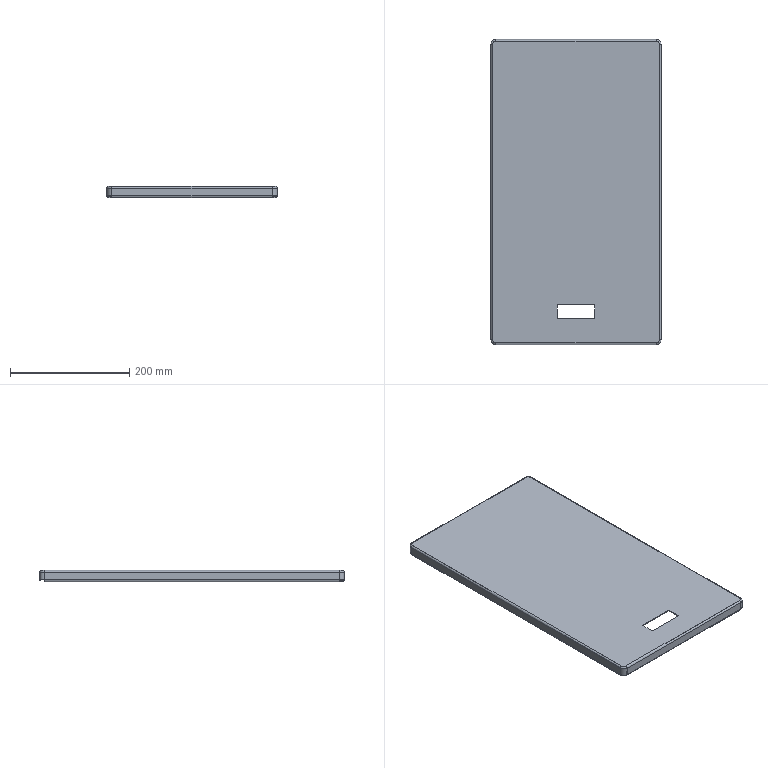Part | STEP file | Front small door panel mating hinge leaf 001 | 1 solid | 114 faces | box 285 x 511 x 19 mm | volume 270507 mm3 | plane 84 | cylinder 22 | torus 8 | commonest cylinder face diameters 3 x7 6 x7 13 x4 16 x4